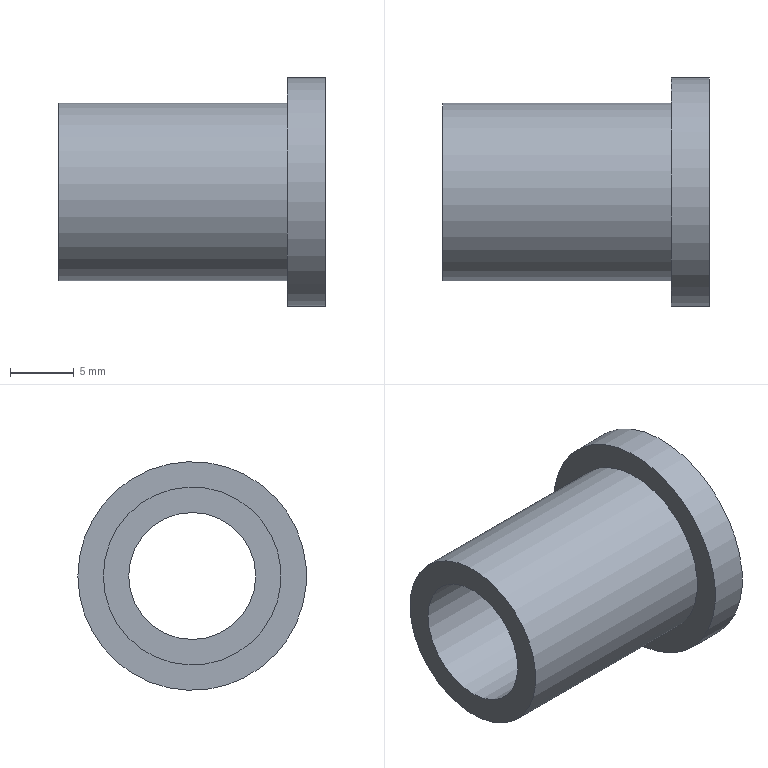Part | STEP file | 1-60L | 1 solid | 6 faces | box 21 x 18 x 18 mm | volume 1885 mm3 | plane 3 | cylinder 3 | commonest cylinder face diameters 10 x1 14 x1 18 x1
STEP:
#1=CARTESIAN_POINT('',(0.,0.,0.));
#2=DIRECTION('',(0.,0.,1.));
#3=DIRECTION('',(1.,0.,0.));
#4=AXIS2_PLACEMENT_3D('',#1,#2,#3);
#5=CARTESIAN_POINT('',(-18.,7.,0.));
#6=VERTEX_POINT('',#5);
#7=CARTESIAN_POINT('',(-18.,0.,0.));
#8=DIRECTION('',(1.,0.,0.));
#9=DIRECTION('',(0.,1.,0.));
#10=AXIS2_PLACEMENT_3D('',#7,#8,#9);
#11=CIRCLE('',#10,7.);
#12=CARTESIAN_POINT('',(-18.,-1.876,0.));
#13=DIRECTION('',(1.,0.,0.));
#14=DIRECTION('',(0.,0.,-1.));
#15=AXIS2_PLACEMENT_3D('',#12,#13,#14);
#16=PLANE('',#15);
#17=CARTESIAN_POINT('',(0.,1.876));
#18=DIRECTION('',(0.,1.));
#19=AXIS2_PLACEMENT_2D('',#17,#18);
#20=CIRCLE('',#19,7.);
#21=(GEOMETRIC_REPRESENTATION_CONTEXT(2)PARAMETRIC_REPRESENTATION_CONTEXT()REPRESENTATION_CONTEXT('',''));
#22=DEFINITIONAL_REPRESENTATION('',(#20),#21);
#23=PCURVE('',#16,#22);
#24=CARTESIAN_POINT('',(0.,0.,0.));
#25=DIRECTION('',(-1.,0.,0.));
#26=DIRECTION('',(0.,1.,0.));
#27=AXIS2_PLACEMENT_3D('',#24,#25,#26);
#28=CYLINDRICAL_SURFACE('',#27,7.);
#29=CARTESIAN_POINT('',(6.283,18.));
#30=DIRECTION('',(-1.,0.));
#31=VECTOR('',#30,1.);
#32=LINE('',#29,#31);
#33=(GEOMETRIC_REPRESENTATION_CONTEXT(2)PARAMETRIC_REPRESENTATION_CONTEXT()REPRESENTATION_CONTEXT('',''));
#34=DEFINITIONAL_REPRESENTATION('',(#32),#33);
#35=PCURVE('',#28,#34);
#36=SURFACE_CURVE('',#11,(#23,#35),.PCURVE_S1.);
#37=EDGE_CURVE('',#6,#6,#36,.T.);
#38=ORIENTED_EDGE('',*,*,#37,.T.);
#39=EDGE_LOOP('',(#38));
#40=FACE_BOUND('',#39,.F.);
#41=CARTESIAN_POINT('',(-18.,5.,0.));
#42=VERTEX_POINT('',#41);
#43=CARTESIAN_POINT('',(-18.,0.,0.));
#44=DIRECTION('',(-1.,0.,0.));
#45=DIRECTION('',(0.,1.,0.));
#46=AXIS2_PLACEMENT_3D('',#43,#44,#45);
#47=CIRCLE('',#46,5.);
#48=CARTESIAN_POINT('',(0.,6.876));
#49=CARTESIAN_POINT('',(8.66,6.876));
#50=CARTESIAN_POINT('',(4.33,-0.6244));
#51=CARTESIAN_POINT('',(0.,-8.124));
#52=CARTESIAN_POINT('',(-4.33,-0.6244));
#53=CARTESIAN_POINT('',(-8.66,6.876));
#54=CARTESIAN_POINT('',(0.,6.876));
#55=(BOUNDED_CURVE()B_SPLINE_CURVE(2,(#48,#49,#50,#51,#52,#53,#54),.UNSPECIFIED.,.T.,.F.)B_SPLINE_CURVE_WITH_KNOTS((1,2,2,2,2,1),(-2.094,0.,2.094,4.189,6.283,8.378),.UNSPECIFIED.)CURVE()GEOMETRIC_REPRESENTATION_ITEM()RATIONAL_B_SPLINE_CURVE((1.,0.5,1.,0.5,1.,0.5,1.))REPRESENTATION_ITEM(''));
#56=(GEOMETRIC_REPRESENTATION_CONTEXT(2)PARAMETRIC_REPRESENTATION_CONTEXT()REPRESENTATION_CONTEXT('',''));
#57=DEFINITIONAL_REPRESENTATION('',(#55),#56);
#58=PCURVE('',#16,#57);
#59=CARTESIAN_POINT('',(3.,0.,0.));
#60=DIRECTION('',(-1.,0.,0.));
#61=DIRECTION('',(0.,1.,0.));
#62=AXIS2_PLACEMENT_3D('',#59,#60,#61);
#63=CYLINDRICAL_SURFACE('',#62,5.);
#64=CARTESIAN_POINT('',(0.,21.));
#65=DIRECTION('',(1.,0.));
#66=VECTOR('',#65,1.);
#67=LINE('',#64,#66);
#68=(GEOMETRIC_REPRESENTATION_CONTEXT(2)PARAMETRIC_REPRESENTATION_CONTEXT()REPRESENTATION_CONTEXT('',''));
#69=DEFINITIONAL_REPRESENTATION('',(#67),#68);
#70=PCURVE('',#63,#69);
#71=SURFACE_CURVE('',#47,(#58,#70),.PCURVE_S1.);
#72=EDGE_CURVE('',#42,#42,#71,.T.);
#73=ORIENTED_EDGE('',*,*,#72,.T.);
#74=EDGE_LOOP('',(#73));
#75=FACE_BOUND('',#74,.F.);
#76=ADVANCED_FACE('',(#40,#75),#16,.F.);
#77=CARTESIAN_POINT('',(0.,7.,0.));
#78=VERTEX_POINT('',#77);
#79=CARTESIAN_POINT('',(0.,7.,0.));
#80=DIRECTION('',(-1.,0.,0.));
#81=VECTOR('',#80,1.);
#82=LINE('',#79,#81);
#83=CARTESIAN_POINT('',(6.283,0.));
#84=DIRECTION('',(0.,1.));
#85=VECTOR('',#84,1.);
#86=LINE('',#83,#85);
#87=(GEOMETRIC_REPRESENTATION_CONTEXT(2)PARAMETRIC_REPRESENTATION_CONTEXT()REPRESENTATION_CONTEXT('',''));
#88=DEFINITIONAL_REPRESENTATION('',(#86),#87);
#89=PCURVE('',#28,#88);
#90=CARTESIAN_POINT('',(0.,0.));
#91=DIRECTION('',(0.,1.));
#92=VECTOR('',#91,1.);
#93=LINE('',#90,#92);
#94=(GEOMETRIC_REPRESENTATION_CONTEXT(2)PARAMETRIC_REPRESENTATION_CONTEXT()REPRESENTATION_CONTEXT('',''));
#95=DEFINITIONAL_REPRESENTATION('',(#93),#94);
#96=PCURVE('',#28,#95);
#97=SEAM_CURVE('',#82,(#89,#96),.PCURVE_S1.);
#98=EDGE_CURVE('',#78,#6,#97,.T.);
#99=ORIENTED_EDGE('',*,*,#98,.T.);
#100=ORIENTED_EDGE('',*,*,#37,.T.);
#101=ORIENTED_EDGE('',*,*,#98,.F.);
#102=CARTESIAN_POINT('',(0.,0.,0.));
#103=DIRECTION('',(1.,0.,0.));
#104=DIRECTION('',(0.,1.,0.));
#105=AXIS2_PLACEMENT_3D('',#102,#103,#104);
#106=CIRCLE('',#105,7.);
#107=CARTESIAN_POINT('',(6.283,0.));
#108=DIRECTION('',(-1.,0.));
#109=VECTOR('',#108,1.);
#110=LINE('',#107,#109);
#111=(GEOMETRIC_REPRESENTATION_CONTEXT(2)PARAMETRIC_REPRESENTATION_CONTEXT()REPRESENTATION_CONTEXT('',''));
#112=DEFINITIONAL_REPRESENTATION('',(#110),#111);
#113=PCURVE('',#28,#112);
#114=CARTESIAN_POINT('',(0.,-2.412,0.));
#115=DIRECTION('',(1.,0.,0.));
#116=DIRECTION('',(0.,0.,-1.));
#117=AXIS2_PLACEMENT_3D('',#114,#115,#116);
#118=PLANE('',#117);
#119=CARTESIAN_POINT('',(0.,2.412));
#120=DIRECTION('',(0.,1.));
#121=AXIS2_PLACEMENT_2D('',#119,#120);
#122=CIRCLE('',#121,7.);
#123=(GEOMETRIC_REPRESENTATION_CONTEXT(2)PARAMETRIC_REPRESENTATION_CONTEXT()REPRESENTATION_CONTEXT('',''));
#124=DEFINITIONAL_REPRESENTATION('',(#122),#123);
#125=PCURVE('',#118,#124);
#126=SURFACE_CURVE('',#106,(#113,#125),.PCURVE_S1.);
#127=EDGE_CURVE('',#78,#78,#126,.T.);
#128=ORIENTED_EDGE('',*,*,#127,.F.);
#129=EDGE_LOOP('',(#99,#100,#101,#128));
#130=FACE_BOUND('',#129,.T.);
#131=ADVANCED_FACE('',(#130),#28,.T.);
#132=ORIENTED_EDGE('',*,*,#72,.F.);
#133=CARTESIAN_POINT('',(3.,5.,0.));
#134=VERTEX_POINT('',#133);
#135=CARTESIAN_POINT('',(-18.,5.,0.));
#136=DIRECTION('',(1.,0.,0.));
#137=VECTOR('',#136,1.);
#138=LINE('',#135,#137);
#139=CARTESIAN_POINT('',(0.,21.));
#140=DIRECTION('',(0.,-1.));
#141=VECTOR('',#140,1.);
#142=LINE('',#139,#141);
#143=(GEOMETRIC_REPRESENTATION_CONTEXT(2)PARAMETRIC_REPRESENTATION_CONTEXT()REPRESENTATION_CONTEXT('',''));
#144=DEFINITIONAL_REPRESENTATION('',(#142),#143);
#145=PCURVE('',#63,#144);
#146=CARTESIAN_POINT('',(6.283,21.));
#147=DIRECTION('',(0.,-1.));
#148=VECTOR('',#147,1.);
#149=LINE('',#146,#148);
#150=(GEOMETRIC_REPRESENTATION_CONTEXT(2)PARAMETRIC_REPRESENTATION_CONTEXT()REPRESENTATION_CONTEXT('',''));
#151=DEFINITIONAL_REPRESENTATION('',(#149),#150);
#152=PCURVE('',#63,#151);
#153=SEAM_CURVE('',#138,(#145,#152),.PCURVE_S1.);
#154=EDGE_CURVE('',#42,#134,#153,.T.);
#155=ORIENTED_EDGE('',*,*,#154,.T.);
#156=CARTESIAN_POINT('',(3.,0.,0.));
#157=DIRECTION('',(-1.,0.,0.));
#158=DIRECTION('',(0.,1.,0.));
#159=AXIS2_PLACEMENT_3D('',#156,#157,#158);
#160=CIRCLE('',#159,5.);
#161=CARTESIAN_POINT('',(0.,0.));
#162=DIRECTION('',(1.,0.));
#163=VECTOR('',#162,1.);
#164=LINE('',#161,#163);
#165=(GEOMETRIC_REPRESENTATION_CONTEXT(2)PARAMETRIC_REPRESENTATION_CONTEXT()REPRESENTATION_CONTEXT('',''));
#166=DEFINITIONAL_REPRESENTATION('',(#164),#165);
#167=PCURVE('',#63,#166);
#168=CARTESIAN_POINT('',(3.,-2.412,0.));
#169=DIRECTION('',(1.,0.,0.));
#170=DIRECTION('',(0.,0.,-1.));
#171=AXIS2_PLACEMENT_3D('',#168,#169,#170);
#172=PLANE('',#171);
#173=CARTESIAN_POINT('',(0.,7.412));
#174=CARTESIAN_POINT('',(8.66,7.412));
#175=CARTESIAN_POINT('',(4.33,-0.08846));
#176=CARTESIAN_POINT('',(0.,-7.588));
#177=CARTESIAN_POINT('',(-4.33,-0.08846));
#178=CARTESIAN_POINT('',(-8.66,7.412));
#179=CARTESIAN_POINT('',(0.,7.412));
#180=(BOUNDED_CURVE()B_SPLINE_CURVE(2,(#173,#174,#175,#176,#177,#178,#179),.UNSPECIFIED.,.T.,.F.)B_SPLINE_CURVE_WITH_KNOTS((1,2,2,2,2,1),(-2.094,0.,2.094,4.189,6.283,8.378),.UNSPECIFIED.)CURVE()GEOMETRIC_REPRESENTATION_ITEM()RATIONAL_B_SPLINE_CURVE((1.,0.5,1.,0.5,1.,0.5,1.))REPRESENTATION_ITEM(''));
#181=(GEOMETRIC_REPRESENTATION_CONTEXT(2)PARAMETRIC_REPRESENTATION_CONTEXT()REPRESENTATION_CONTEXT('',''));
#182=DEFINITIONAL_REPRESENTATION('',(#180),#181);
#183=PCURVE('',#172,#182);
#184=SURFACE_CURVE('',#160,(#167,#183),.PCURVE_S1.);
#185=EDGE_CURVE('',#134,#134,#184,.T.);
#186=ORIENTED_EDGE('',*,*,#185,.T.);
#187=ORIENTED_EDGE('',*,*,#154,.F.);
#188=EDGE_LOOP('',(#132,#155,#186,#187));
#189=FACE_BOUND('',#188,.F.);
#190=ADVANCED_FACE('',(#189),#63,.F.);
#191=CARTESIAN_POINT('',(0.,9.,0.));
#192=VERTEX_POINT('',#191);
#193=CARTESIAN_POINT('',(0.,0.,0.));
#194=DIRECTION('',(1.,0.,0.));
#195=DIRECTION('',(0.,1.,0.));
#196=AXIS2_PLACEMENT_3D('',#193,#194,#195);
#197=CIRCLE('',#196,9.);
#198=CARTESIAN_POINT('',(0.,2.412));
#199=DIRECTION('',(0.,1.));
#200=AXIS2_PLACEMENT_2D('',#198,#199);
#201=CIRCLE('',#200,9.);
#202=(GEOMETRIC_REPRESENTATION_CONTEXT(2)PARAMETRIC_REPRESENTATION_CONTEXT()REPRESENTATION_CONTEXT('',''));
#203=DEFINITIONAL_REPRESENTATION('',(#201),#202);
#204=PCURVE('',#118,#203);
#205=CARTESIAN_POINT('',(0.,0.,0.));
#206=DIRECTION('',(1.,0.,0.));
#207=DIRECTION('',(0.,1.,0.));
#208=AXIS2_PLACEMENT_3D('',#205,#206,#207);
#209=CYLINDRICAL_SURFACE('',#208,9.);
#210=CARTESIAN_POINT('',(0.,0.));
#211=DIRECTION('',(1.,0.));
#212=VECTOR('',#211,1.);
#213=LINE('',#210,#212);
#214=(GEOMETRIC_REPRESENTATION_CONTEXT(2)PARAMETRIC_REPRESENTATION_CONTEXT()REPRESENTATION_CONTEXT('',''));
#215=DEFINITIONAL_REPRESENTATION('',(#213),#214);
#216=PCURVE('',#209,#215);
#217=SURFACE_CURVE('',#197,(#204,#216),.PCURVE_S1.);
#218=EDGE_CURVE('',#192,#192,#217,.T.);
#219=ORIENTED_EDGE('',*,*,#218,.T.);
#220=EDGE_LOOP('',(#219));
#221=FACE_BOUND('',#220,.F.);
#222=ORIENTED_EDGE('',*,*,#127,.F.);
#223=EDGE_LOOP('',(#222));
#224=FACE_BOUND('',#223,.F.);
#225=ADVANCED_FACE('',(#221,#224),#118,.F.);
#226=ORIENTED_EDGE('',*,*,#218,.T.);
#227=CARTESIAN_POINT('',(3.,9.,0.));
#228=VERTEX_POINT('',#227);
#229=CARTESIAN_POINT('',(0.,9.,0.));
#230=DIRECTION('',(1.,0.,0.));
#231=VECTOR('',#230,1.);
#232=LINE('',#229,#231);
#233=CARTESIAN_POINT('',(6.283,0.));
#234=DIRECTION('',(0.,1.));
#235=VECTOR('',#234,1.);
#236=LINE('',#233,#235);
#237=(GEOMETRIC_REPRESENTATION_CONTEXT(2)PARAMETRIC_REPRESENTATION_CONTEXT()REPRESENTATION_CONTEXT('',''));
#238=DEFINITIONAL_REPRESENTATION('',(#236),#237);
#239=PCURVE('',#209,#238);
#240=CARTESIAN_POINT('',(0.,0.));
#241=DIRECTION('',(0.,1.));
#242=VECTOR('',#241,1.);
#243=LINE('',#240,#242);
#244=(GEOMETRIC_REPRESENTATION_CONTEXT(2)PARAMETRIC_REPRESENTATION_CONTEXT()REPRESENTATION_CONTEXT('',''));
#245=DEFINITIONAL_REPRESENTATION('',(#243),#244);
#246=PCURVE('',#209,#245);
#247=SEAM_CURVE('',#232,(#239,#246),.PCURVE_S1.);
#248=EDGE_CURVE('',#192,#228,#247,.T.);
#249=ORIENTED_EDGE('',*,*,#248,.T.);
#250=CARTESIAN_POINT('',(3.,0.,0.));
#251=DIRECTION('',(1.,0.,0.));
#252=DIRECTION('',(0.,1.,0.));
#253=AXIS2_PLACEMENT_3D('',#250,#251,#252);
#254=CIRCLE('',#253,9.);
#255=CARTESIAN_POINT('',(0.,3.));
#256=DIRECTION('',(1.,0.));
#257=VECTOR('',#256,1.);
#258=LINE('',#255,#257);
#259=(GEOMETRIC_REPRESENTATION_CONTEXT(2)PARAMETRIC_REPRESENTATION_CONTEXT()REPRESENTATION_CONTEXT('',''));
#260=DEFINITIONAL_REPRESENTATION('',(#258),#259);
#261=PCURVE('',#209,#260);
#262=CARTESIAN_POINT('',(0.,2.412));
#263=DIRECTION('',(0.,1.));
#264=AXIS2_PLACEMENT_2D('',#262,#263);
#265=CIRCLE('',#264,9.);
#266=(GEOMETRIC_REPRESENTATION_CONTEXT(2)PARAMETRIC_REPRESENTATION_CONTEXT()REPRESENTATION_CONTEXT('',''));
#267=DEFINITIONAL_REPRESENTATION('',(#265),#266);
#268=PCURVE('',#172,#267);
#269=SURFACE_CURVE('',#254,(#261,#268),.PCURVE_S1.);
#270=EDGE_CURVE('',#228,#228,#269,.T.);
#271=ORIENTED_EDGE('',*,*,#270,.F.);
#272=ORIENTED_EDGE('',*,*,#248,.F.);
#273=EDGE_LOOP('',(#226,#249,#271,#272));
#274=FACE_BOUND('',#273,.T.);
#275=ADVANCED_FACE('',(#274),#209,.T.);
#276=ORIENTED_EDGE('',*,*,#270,.T.);
#277=EDGE_LOOP('',(#276));
#278=FACE_BOUND('',#277,.T.);
#279=ORIENTED_EDGE('',*,*,#185,.T.);
#280=EDGE_LOOP('',(#279));
#281=FACE_BOUND('',#280,.T.);
#282=ADVANCED_FACE('',(#278,#281),#172,.T.);
#283=CLOSED_SHELL('',(#76,#131,#190,#225,#275,#282));
#284=MANIFOLD_SOLID_BREP('',#283);
#285=(LENGTH_UNIT()NAMED_UNIT(*)SI_UNIT(.MILLI.,.METRE.));
#286=UNCERTAINTY_MEASURE_WITH_UNIT(LENGTH_MEASURE(0.0000001),#285,'','');
#287=(NAMED_UNIT(*)PLANE_ANGLE_UNIT()SI_UNIT($,.RADIAN.));
#288=(NAMED_UNIT(*)SI_UNIT($,.STERADIAN.)SOLID_ANGLE_UNIT());
#289=(GEOMETRIC_REPRESENTATION_CONTEXT(3)GLOBAL_UNCERTAINTY_ASSIGNED_CONTEXT((#286))GLOBAL_UNIT_ASSIGNED_CONTEXT((#285,#287,#288))REPRESENTATION_CONTEXT('',''));
#290=ADVANCED_BREP_SHAPE_REPRESENTATION('',(#4,#284),#289);